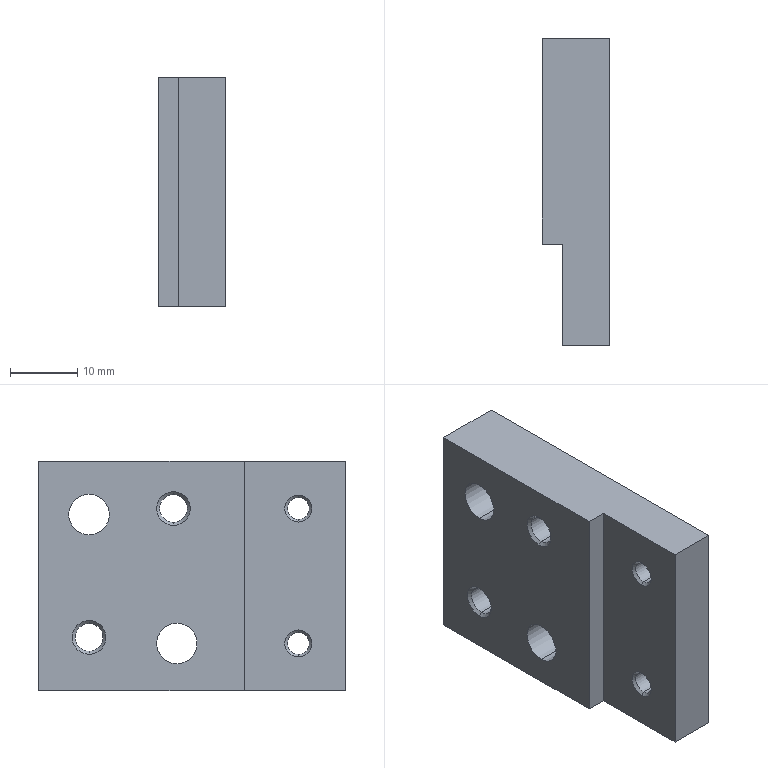Part | SolidWorks | features MirrorStock 1 | 1 solid | 28 faces | box 10 x 45.5 x 34 mm | volume 12986 mm3 | cylinder 12 | cone 8 | plane 8 | commonest cylinder face diameters 3.242 x4 4.134 x4 6 x4
STEP:
#1=CARTESIAN_POINT('',(-38.,7.5,-11.167));
#2=VERTEX_POINT('',#1);
#3=CARTESIAN_POINT('',(-38.,7.5,-7.033));
#4=VERTEX_POINT('',#3);
#5=CARTESIAN_POINT('',(-38.,7.5,-9.1));
#6=DIRECTION('',(-1.,0.,0.));
#7=DIRECTION('',(0.,0.,1.));
#8=AXIS2_PLACEMENT_3D('',#5,#6,#7);
#9=CIRCLE('',#8,2.067);
#10=EDGE_CURVE('',#2,#4,#9,.T.);
#11=ORIENTED_EDGE('',*,*,#10,.F.);
#12=CARTESIAN_POINT('',(-47.567,7.5,-11.167));
#13=VERTEX_POINT('',#12);
#14=CARTESIAN_POINT('',(-38.,7.5,-11.167));
#15=DIRECTION('',(-1.,0.,0.));
#16=VECTOR('',#15,1000.);
#17=LINE('',#14,#16);
#18=EDGE_CURVE('',#2,#13,#17,.T.);
#19=ORIENTED_EDGE('',*,*,#18,.T.);
#20=CARTESIAN_POINT('',(-47.567,7.5,-7.033));
#21=VERTEX_POINT('',#20);
#22=CARTESIAN_POINT('',(-47.567,7.5,-9.1));
#23=DIRECTION('',(-1.,0.,0.));
#24=DIRECTION('',(0.,0.,1.));
#25=AXIS2_PLACEMENT_3D('',#22,#23,#24);
#26=CIRCLE('',#25,2.067);
#27=EDGE_CURVE('',#13,#21,#26,.T.);
#28=ORIENTED_EDGE('',*,*,#27,.T.);
#29=CARTESIAN_POINT('',(-38.,7.5,-7.033));
#30=DIRECTION('',(-1.,0.,0.));
#31=VECTOR('',#30,1000.);
#32=LINE('',#29,#31);
#33=EDGE_CURVE('',#4,#21,#32,.T.);
#34=ORIENTED_EDGE('',*,*,#33,.F.);
#35=EDGE_LOOP('',(#11,#19,#28,#34));
#36=FACE_OUTER_BOUND('',#35,.T.);
#37=CARTESIAN_POINT('',(-38.,7.5,-9.1));
#38=DIRECTION('',(-1.,0.,0.));
#39=DIRECTION('',(0.,0.,1.));
#40=AXIS2_PLACEMENT_3D('',#37,#38,#39);
#41=CYLINDRICAL_SURFACE('',#40,2.067);
#42=ADVANCED_FACE('',(#36),#41,.F.);
#43=CARTESIAN_POINT('',(-47.567,7.5,-9.1));
#44=DIRECTION('',(-1.,0.,0.));
#45=DIRECTION('',(0.,0.,1.));
#46=AXIS2_PLACEMENT_3D('',#43,#44,#45);
#47=CIRCLE('',#46,2.067);
#48=EDGE_CURVE('',#21,#13,#47,.T.);
#49=ORIENTED_EDGE('',*,*,#48,.F.);
#50=CARTESIAN_POINT('',(-48.,7.5,-6.6));
#51=VERTEX_POINT('',#50);
#52=CARTESIAN_POINT('',(-48.,7.5,-6.6));
#53=DIRECTION('',(-0.7071,0.,0.7071));
#54=VECTOR('',#53,1000.);
#55=LINE('',#52,#54);
#56=EDGE_CURVE('',#21,#51,#55,.T.);
#57=ORIENTED_EDGE('',*,*,#56,.T.);
#58=CARTESIAN_POINT('',(-48.,7.5,-11.6));
#59=VERTEX_POINT('',#58);
#60=CARTESIAN_POINT('',(-48.,7.5,-9.1));
#61=DIRECTION('',(-1.,0.,0.));
#62=DIRECTION('',(0.,0.,1.));
#63=AXIS2_PLACEMENT_3D('',#60,#61,#62);
#64=CIRCLE('',#63,2.5);
#65=EDGE_CURVE('',#51,#59,#64,.T.);
#66=ORIENTED_EDGE('',*,*,#65,.T.);
#67=CARTESIAN_POINT('',(-48.,7.5,-11.6));
#68=DIRECTION('',(-0.7071,0.,-0.7071));
#69=VECTOR('',#68,1000.);
#70=LINE('',#67,#69);
#71=EDGE_CURVE('',#13,#59,#70,.T.);
#72=ORIENTED_EDGE('',*,*,#71,.F.);
#73=EDGE_LOOP('',(#49,#57,#66,#72));
#74=FACE_OUTER_BOUND('',#73,.T.);
#75=CARTESIAN_POINT('',(-48.,7.5,-9.1));
#76=DIRECTION('',(-1.,0.,0.));
#77=DIRECTION('',(0.,0.,-1.));
#78=AXIS2_PLACEMENT_3D('',#75,#76,#77);
#79=CONICAL_SURFACE('',#78,2.5,0.7854);
#80=ADVANCED_FACE('',(#74),#79,.F.);
#81=CARTESIAN_POINT('',(-38.,-5.,7.933));
#82=VERTEX_POINT('',#81);
#83=CARTESIAN_POINT('',(-38.,-5.,12.067));
#84=VERTEX_POINT('',#83);
#85=CARTESIAN_POINT('',(-38.,-5.,10.));
#86=DIRECTION('',(-1.,0.,0.));
#87=DIRECTION('',(0.,0.,1.));
#88=AXIS2_PLACEMENT_3D('',#85,#86,#87);
#89=CIRCLE('',#88,2.067);
#90=EDGE_CURVE('',#82,#84,#89,.T.);
#91=ORIENTED_EDGE('',*,*,#90,.F.);
#92=CARTESIAN_POINT('',(-47.567,-5.,7.933));
#93=VERTEX_POINT('',#92);
#94=CARTESIAN_POINT('',(-38.,-5.,7.933));
#95=DIRECTION('',(-1.,0.,0.));
#96=VECTOR('',#95,1000.);
#97=LINE('',#94,#96);
#98=EDGE_CURVE('',#82,#93,#97,.T.);
#99=ORIENTED_EDGE('',*,*,#98,.T.);
#100=CARTESIAN_POINT('',(-47.567,-5.,12.067));
#101=VERTEX_POINT('',#100);
#102=CARTESIAN_POINT('',(-47.567,-5.,10.));
#103=DIRECTION('',(-1.,0.,0.));
#104=DIRECTION('',(0.,0.,1.));
#105=AXIS2_PLACEMENT_3D('',#102,#103,#104);
#106=CIRCLE('',#105,2.067);
#107=EDGE_CURVE('',#93,#101,#106,.T.);
#108=ORIENTED_EDGE('',*,*,#107,.T.);
#109=CARTESIAN_POINT('',(-38.,-5.,12.067));
#110=DIRECTION('',(-1.,0.,0.));
#111=VECTOR('',#110,1000.);
#112=LINE('',#109,#111);
#113=EDGE_CURVE('',#84,#101,#112,.T.);
#114=ORIENTED_EDGE('',*,*,#113,.F.);
#115=EDGE_LOOP('',(#91,#99,#108,#114));
#116=FACE_OUTER_BOUND('',#115,.T.);
#117=CARTESIAN_POINT('',(-38.,-5.,10.));
#118=DIRECTION('',(-1.,0.,0.));
#119=DIRECTION('',(0.,0.,1.));
#120=AXIS2_PLACEMENT_3D('',#117,#118,#119);
#121=CYLINDRICAL_SURFACE('',#120,2.067);
#122=ADVANCED_FACE('',(#116),#121,.F.);
#123=CARTESIAN_POINT('',(-47.567,-5.,10.));
#124=DIRECTION('',(-1.,0.,0.));
#125=DIRECTION('',(0.,0.,1.));
#126=AXIS2_PLACEMENT_3D('',#123,#124,#125);
#127=CIRCLE('',#126,2.067);
#128=EDGE_CURVE('',#101,#93,#127,.T.);
#129=ORIENTED_EDGE('',*,*,#128,.F.);
#130=CARTESIAN_POINT('',(-48.,-5.,12.5));
#131=VERTEX_POINT('',#130);
#132=CARTESIAN_POINT('',(-48.,-5.,12.5));
#133=DIRECTION('',(-0.7071,0.,0.7071));
#134=VECTOR('',#133,1000.);
#135=LINE('',#132,#134);
#136=EDGE_CURVE('',#101,#131,#135,.T.);
#137=ORIENTED_EDGE('',*,*,#136,.T.);
#138=CARTESIAN_POINT('',(-48.,-5.,7.5));
#139=VERTEX_POINT('',#138);
#140=CARTESIAN_POINT('',(-48.,-5.,10.));
#141=DIRECTION('',(-1.,0.,0.));
#142=DIRECTION('',(0.,0.,1.));
#143=AXIS2_PLACEMENT_3D('',#140,#141,#142);
#144=CIRCLE('',#143,2.5);
#145=EDGE_CURVE('',#131,#139,#144,.T.);
#146=ORIENTED_EDGE('',*,*,#145,.T.);
#147=CARTESIAN_POINT('',(-48.,-5.,7.5));
#148=DIRECTION('',(-0.7071,0.,-0.7071));
#149=VECTOR('',#148,1000.);
#150=LINE('',#147,#149);
#151=EDGE_CURVE('',#93,#139,#150,.T.);
#152=ORIENTED_EDGE('',*,*,#151,.F.);
#153=EDGE_LOOP('',(#129,#137,#146,#152));
#154=FACE_OUTER_BOUND('',#153,.T.);
#155=CARTESIAN_POINT('',(-48.,-5.,10.));
#156=DIRECTION('',(-1.,0.,0.));
#157=DIRECTION('',(0.,0.,-1.));
#158=AXIS2_PLACEMENT_3D('',#155,#156,#157);
#159=CONICAL_SURFACE('',#158,2.5,0.7854);
#160=ADVANCED_FACE('',(#154),#159,.F.);
#161=CARTESIAN_POINT('',(-38.,-23.5,11.621));
#162=VERTEX_POINT('',#161);
#163=CARTESIAN_POINT('',(-38.,-23.5,8.379));
#164=VERTEX_POINT('',#163);
#165=CARTESIAN_POINT('',(-38.,-23.5,10.));
#166=DIRECTION('',(1.,0.,0.));
#167=DIRECTION('',(0.,0.,1.));
#168=AXIS2_PLACEMENT_3D('',#165,#166,#167);
#169=CIRCLE('',#168,1.621);
#170=EDGE_CURVE('',#162,#164,#169,.T.);
#171=ORIENTED_EDGE('',*,*,#170,.T.);
#172=CARTESIAN_POINT('',(-44.621,-23.5,8.379));
#173=VERTEX_POINT('',#172);
#174=CARTESIAN_POINT('',(-35.,-23.5,8.379));
#175=DIRECTION('',(-1.,0.,0.));
#176=VECTOR('',#175,1000.);
#177=LINE('',#174,#176);
#178=EDGE_CURVE('',#164,#173,#177,.T.);
#179=ORIENTED_EDGE('',*,*,#178,.T.);
#180=CARTESIAN_POINT('',(-44.621,-23.5,11.621));
#181=VERTEX_POINT('',#180);
#182=CARTESIAN_POINT('',(-44.621,-23.5,10.));
#183=DIRECTION('',(-1.,0.,0.));
#184=DIRECTION('',(0.,0.,1.));
#185=AXIS2_PLACEMENT_3D('',#182,#183,#184);
#186=CIRCLE('',#185,1.621);
#187=EDGE_CURVE('',#173,#181,#186,.T.);
#188=ORIENTED_EDGE('',*,*,#187,.T.);
#189=CARTESIAN_POINT('',(-35.,-23.5,11.621));
#190=DIRECTION('',(-1.,0.,0.));
#191=VECTOR('',#190,1000.);
#192=LINE('',#189,#191);
#193=EDGE_CURVE('',#162,#181,#192,.T.);
#194=ORIENTED_EDGE('',*,*,#193,.F.);
#195=EDGE_LOOP('',(#171,#179,#188,#194));
#196=FACE_OUTER_BOUND('',#195,.T.);
#197=CARTESIAN_POINT('',(-35.,-23.5,10.));
#198=DIRECTION('',(-1.,0.,0.));
#199=DIRECTION('',(0.,0.,1.));
#200=AXIS2_PLACEMENT_3D('',#197,#198,#199);
#201=CYLINDRICAL_SURFACE('',#200,1.621);
#202=ADVANCED_FACE('',(#196),#201,.F.);
#203=CARTESIAN_POINT('',(-44.621,-23.5,10.));
#204=DIRECTION('',(-1.,0.,0.));
#205=DIRECTION('',(0.,0.,1.));
#206=AXIS2_PLACEMENT_3D('',#203,#204,#205);
#207=CIRCLE('',#206,1.621);
#208=EDGE_CURVE('',#181,#173,#207,.T.);
#209=ORIENTED_EDGE('',*,*,#208,.F.);
#210=CARTESIAN_POINT('',(-45.,-23.5,12.));
#211=VERTEX_POINT('',#210);
#212=CARTESIAN_POINT('',(-45.,-23.5,12.));
#213=DIRECTION('',(-0.7071,0.,0.7071));
#214=VECTOR('',#213,1000.);
#215=LINE('',#212,#214);
#216=EDGE_CURVE('',#181,#211,#215,.T.);
#217=ORIENTED_EDGE('',*,*,#216,.T.);
#218=CARTESIAN_POINT('',(-45.,-23.5,8.));
#219=VERTEX_POINT('',#218);
#220=CARTESIAN_POINT('',(-45.,-23.5,10.));
#221=DIRECTION('',(-1.,0.,0.));
#222=DIRECTION('',(0.,0.,1.));
#223=AXIS2_PLACEMENT_3D('',#220,#221,#222);
#224=CIRCLE('',#223,2.);
#225=EDGE_CURVE('',#211,#219,#224,.T.);
#226=ORIENTED_EDGE('',*,*,#225,.T.);
#227=CARTESIAN_POINT('',(-45.,-23.5,8.));
#228=DIRECTION('',(-0.7071,0.,-0.7071));
#229=VECTOR('',#228,1000.);
#230=LINE('',#227,#229);
#231=EDGE_CURVE('',#173,#219,#230,.T.);
#232=ORIENTED_EDGE('',*,*,#231,.F.);
#233=EDGE_LOOP('',(#209,#217,#226,#232));
#234=FACE_OUTER_BOUND('',#233,.T.);
#235=CARTESIAN_POINT('',(-45.,-23.5,10.));
#236=DIRECTION('',(-1.,0.,0.));
#237=DIRECTION('',(0.,0.,-1.));
#238=AXIS2_PLACEMENT_3D('',#235,#236,#237);
#239=CONICAL_SURFACE('',#238,2.,0.7854);
#240=ADVANCED_FACE('',(#234),#239,.F.);
#241=CARTESIAN_POINT('',(-44.621,-23.5,-8.379));
#242=VERTEX_POINT('',#241);
#243=CARTESIAN_POINT('',(-44.621,-23.5,-11.621));
#244=VERTEX_POINT('',#243);
#245=CARTESIAN_POINT('',(-44.621,-23.5,-10.));
#246=DIRECTION('',(-1.,0.,0.));
#247=DIRECTION('',(0.,0.,1.));
#248=AXIS2_PLACEMENT_3D('',#245,#246,#247);
#249=CIRCLE('',#248,1.621);
#250=EDGE_CURVE('',#242,#244,#249,.T.);
#251=ORIENTED_EDGE('',*,*,#250,.F.);
#252=CARTESIAN_POINT('',(-45.,-23.5,-8.));
#253=VERTEX_POINT('',#252);
#254=CARTESIAN_POINT('',(-45.,-23.5,-8.));
#255=DIRECTION('',(-0.7071,0.,0.7071));
#256=VECTOR('',#255,1000.);
#257=LINE('',#254,#256);
#258=EDGE_CURVE('',#242,#253,#257,.T.);
#259=ORIENTED_EDGE('',*,*,#258,.T.);
#260=CARTESIAN_POINT('',(-45.,-23.5,-12.));
#261=VERTEX_POINT('',#260);
#262=CARTESIAN_POINT('',(-45.,-23.5,-10.));
#263=DIRECTION('',(-1.,0.,0.));
#264=DIRECTION('',(0.,0.,1.));
#265=AXIS2_PLACEMENT_3D('',#262,#263,#264);
#266=CIRCLE('',#265,2.);
#267=EDGE_CURVE('',#253,#261,#266,.T.);
#268=ORIENTED_EDGE('',*,*,#267,.T.);
#269=CARTESIAN_POINT('',(-45.,-23.5,-12.));
#270=DIRECTION('',(-0.7071,0.,-0.7071));
#271=VECTOR('',#270,1000.);
#272=LINE('',#269,#271);
#273=EDGE_CURVE('',#244,#261,#272,.T.);
#274=ORIENTED_EDGE('',*,*,#273,.F.);
#275=EDGE_LOOP('',(#251,#259,#268,#274));
#276=FACE_OUTER_BOUND('',#275,.T.);
#277=CARTESIAN_POINT('',(-45.,-23.5,-10.));
#278=DIRECTION('',(-1.,0.,0.));
#279=DIRECTION('',(0.,0.,-1.));
#280=AXIS2_PLACEMENT_3D('',#277,#278,#279);
#281=CONICAL_SURFACE('',#280,2.,0.7854);
#282=ADVANCED_FACE('',(#276),#281,.F.);
#283=CARTESIAN_POINT('',(-38.,-5.5,-13.));
#284=VERTEX_POINT('',#283);
#285=CARTESIAN_POINT('',(-38.,-5.5,-7.));
#286=VERTEX_POINT('',#285);
#287=CARTESIAN_POINT('',(-38.,-5.5,-10.));
#288=DIRECTION('',(-1.,0.,0.));
#289=DIRECTION('',(0.,0.,1.));
#290=AXIS2_PLACEMENT_3D('',#287,#288,#289);
#291=CIRCLE('',#290,3.);
#292=EDGE_CURVE('',#284,#286,#291,.T.);
#293=ORIENTED_EDGE('',*,*,#292,.F.);
#294=CARTESIAN_POINT('',(-48.,-5.5,-13.));
#295=VERTEX_POINT('',#294);
#296=CARTESIAN_POINT('',(-100.,-5.5,-13.));
#297=DIRECTION('',(-1.,0.,0.));
#298=VECTOR('',#297,1000.);
#299=LINE('',#296,#298);
#300=EDGE_CURVE('',#284,#295,#299,.T.);
#301=ORIENTED_EDGE('',*,*,#300,.T.);
#302=CARTESIAN_POINT('',(-48.,-5.5,-7.));
#303=VERTEX_POINT('',#302);
#304=CARTESIAN_POINT('',(-48.,-5.5,-10.));
#305=DIRECTION('',(-1.,0.,0.));
#306=DIRECTION('',(0.,0.,1.));
#307=AXIS2_PLACEMENT_3D('',#304,#305,#306);
#308=CIRCLE('',#307,3.);
#309=EDGE_CURVE('',#295,#303,#308,.T.);
#310=ORIENTED_EDGE('',*,*,#309,.T.);
#311=CARTESIAN_POINT('',(-100.,-5.5,-7.));
#312=DIRECTION('',(-1.,0.,0.));
#313=VECTOR('',#312,1000.);
#314=LINE('',#311,#313);
#315=EDGE_CURVE('',#286,#303,#314,.T.);
#316=ORIENTED_EDGE('',*,*,#315,.F.);
#317=EDGE_LOOP('',(#293,#301,#310,#316));
#318=FACE_OUTER_BOUND('',#317,.T.);
#319=CARTESIAN_POINT('',(-100.,-5.5,-10.));
#320=DIRECTION('',(-1.,0.,0.));
#321=DIRECTION('',(0.,0.,1.));
#322=AXIS2_PLACEMENT_3D('',#319,#320,#321);
#323=CYLINDRICAL_SURFACE('',#322,3.);
#324=ADVANCED_FACE('',(#318),#323,.F.);
#325=CARTESIAN_POINT('',(-38.,7.5,6.1));
#326=VERTEX_POINT('',#325);
#327=CARTESIAN_POINT('',(-38.,7.5,12.1));
#328=VERTEX_POINT('',#327);
#329=CARTESIAN_POINT('',(-38.,7.5,9.1));
#330=DIRECTION('',(-1.,0.,0.));
#331=DIRECTION('',(0.,0.,1.));
#332=AXIS2_PLACEMENT_3D('',#329,#330,#331);
#333=CIRCLE('',#332,3.);
#334=EDGE_CURVE('',#326,#328,#333,.T.);
#335=ORIENTED_EDGE('',*,*,#334,.F.);
#336=CARTESIAN_POINT('',(-48.,7.5,6.1));
#337=VERTEX_POINT('',#336);
#338=CARTESIAN_POINT('',(-100.,7.5,6.1));
#339=DIRECTION('',(-1.,0.,0.));
#340=VECTOR('',#339,1000.);
#341=LINE('',#338,#340);
#342=EDGE_CURVE('',#326,#337,#341,.T.);
#343=ORIENTED_EDGE('',*,*,#342,.T.);
#344=CARTESIAN_POINT('',(-48.,7.5,12.1));
#345=VERTEX_POINT('',#344);
#346=CARTESIAN_POINT('',(-48.,7.5,9.1));
#347=DIRECTION('',(-1.,0.,0.));
#348=DIRECTION('',(0.,0.,1.));
#349=AXIS2_PLACEMENT_3D('',#346,#347,#348);
#350=CIRCLE('',#349,3.);
#351=EDGE_CURVE('',#337,#345,#350,.T.);
#352=ORIENTED_EDGE('',*,*,#351,.T.);
#353=CARTESIAN_POINT('',(-100.,7.5,12.1));
#354=DIRECTION('',(-1.,0.,0.));
#355=VECTOR('',#354,1000.);
#356=LINE('',#353,#355);
#357=EDGE_CURVE('',#328,#345,#356,.T.);
#358=ORIENTED_EDGE('',*,*,#357,.F.);
#359=EDGE_LOOP('',(#335,#343,#352,#358));
#360=FACE_OUTER_BOUND('',#359,.T.);
#361=CARTESIAN_POINT('',(-100.,7.5,9.1));
#362=DIRECTION('',(-1.,0.,0.));
#363=DIRECTION('',(0.,0.,1.));
#364=AXIS2_PLACEMENT_3D('',#361,#362,#363);
#365=CYLINDRICAL_SURFACE('',#364,3.);
#366=ADVANCED_FACE('',(#360),#365,.F.);
#367=CARTESIAN_POINT('',(-38.,-23.5,-8.379));
#368=VERTEX_POINT('',#367);
#369=CARTESIAN_POINT('',(-38.,-23.5,-11.621));
#370=VERTEX_POINT('',#369);
#371=CARTESIAN_POINT('',(-38.,-23.5,-10.));
#372=DIRECTION('',(1.,0.,0.));
#373=DIRECTION('',(0.,0.,1.));
#374=AXIS2_PLACEMENT_3D('',#371,#372,#373);
#375=CIRCLE('',#374,1.621);
#376=EDGE_CURVE('',#368,#370,#375,.T.);
#377=ORIENTED_EDGE('',*,*,#376,.T.);
#378=CARTESIAN_POINT('',(-35.,-23.5,-11.621));
#379=DIRECTION('',(-1.,0.,0.));
#380=VECTOR('',#379,1000.);
#381=LINE('',#378,#380);
#382=EDGE_CURVE('',#370,#244,#381,.T.);
#383=ORIENTED_EDGE('',*,*,#382,.T.);
#384=CARTESIAN_POINT('',(-44.621,-23.5,-10.));
#385=DIRECTION('',(-1.,0.,0.));
#386=DIRECTION('',(0.,0.,1.));
#387=AXIS2_PLACEMENT_3D('',#384,#385,#386);
#388=CIRCLE('',#387,1.621);
#389=EDGE_CURVE('',#244,#242,#388,.T.);
#390=ORIENTED_EDGE('',*,*,#389,.T.);
#391=CARTESIAN_POINT('',(-35.,-23.5,-8.379));
#392=DIRECTION('',(-1.,0.,0.));
#393=VECTOR('',#392,1000.);
#394=LINE('',#391,#393);
#395=EDGE_CURVE('',#368,#242,#394,.T.);
#396=ORIENTED_EDGE('',*,*,#395,.F.);
#397=EDGE_LOOP('',(#377,#383,#390,#396));
#398=FACE_OUTER_BOUND('',#397,.T.);
#399=CARTESIAN_POINT('',(-35.,-23.5,-10.));
#400=DIRECTION('',(-1.,0.,0.));
#401=DIRECTION('',(0.,0.,1.));
#402=AXIS2_PLACEMENT_3D('',#399,#400,#401);
#403=CYLINDRICAL_SURFACE('',#402,1.621);
#404=ADVANCED_FACE('',(#398),#403,.F.);
#405=ORIENTED_EDGE('',*,*,#382,.F.);
#406=CARTESIAN_POINT('',(-38.,-23.5,-10.));
#407=DIRECTION('',(1.,0.,0.));
#408=DIRECTION('',(0.,0.,1.));
#409=AXIS2_PLACEMENT_3D('',#406,#407,#408);
#410=CIRCLE('',#409,1.621);
#411=EDGE_CURVE('',#370,#368,#410,.T.);
#412=ORIENTED_EDGE('',*,*,#411,.T.);
#413=ORIENTED_EDGE('',*,*,#395,.T.);
#414=ORIENTED_EDGE('',*,*,#250,.T.);
#415=EDGE_LOOP('',(#405,#412,#413,#414));
#416=FACE_OUTER_BOUND('',#415,.T.);
#417=CARTESIAN_POINT('',(-35.,-23.5,-10.));
#418=DIRECTION('',(-1.,0.,0.));
#419=DIRECTION('',(0.,0.,1.));
#420=AXIS2_PLACEMENT_3D('',#417,#418,#419);
#421=CYLINDRICAL_SURFACE('',#420,1.621);
#422=ADVANCED_FACE('',(#416),#421,.F.);
#423=CARTESIAN_POINT('',(-45.,-30.5,-17.));
#424=VERTEX_POINT('',#423);
#425=CARTESIAN_POINT('',(-45.,-30.5,17.));
#426=VERTEX_POINT('',#425);
#427=CARTESIAN_POINT('',(-45.,-30.5,-17.));
#428=DIRECTION('',(0.,0.,1.));
#429=VECTOR('',#428,1000.);
#430=LINE('',#427,#429);
#431=EDGE_CURVE('',#424,#426,#430,.T.);
#432=ORIENTED_EDGE('',*,*,#431,.F.);
#433=CARTESIAN_POINT('',(-38.,-30.5,-17.));
#434=VERTEX_POINT('',#433);
#435=CARTESIAN_POINT('',(-48.,-30.5,-17.));
#436=DIRECTION('',(1.,0.,0.));
#437=VECTOR('',#436,1000.);
#438=LINE('',#435,#437);
#439=EDGE_CURVE('',#424,#434,#438,.T.);
#440=ORIENTED_EDGE('',*,*,#439,.T.);
#441=CARTESIAN_POINT('',(-38.,-30.5,17.));
#442=VERTEX_POINT('',#441);
#443=CARTESIAN_POINT('',(-38.,-30.5,-17.));
#444=DIRECTION('',(0.,0.,1.));
#445=VECTOR('',#444,1000.);
#446=LINE('',#443,#445);
#447=EDGE_CURVE('',#434,#442,#446,.T.);
#448=ORIENTED_EDGE('',*,*,#447,.T.);
#449=CARTESIAN_POINT('',(-48.,-30.5,17.));
#450=DIRECTION('',(1.,0.,0.));
#451=VECTOR('',#450,1000.);
#452=LINE('',#449,#451);
#453=EDGE_CURVE('',#426,#442,#452,.T.);
#454=ORIENTED_EDGE('',*,*,#453,.F.);
#455=EDGE_LOOP('',(#432,#440,#448,#454));
#456=FACE_OUTER_BOUND('',#455,.T.);
#457=CARTESIAN_POINT('',(-48.,-30.5,-17.));
#458=DIRECTION('',(0.,-1.,0.));
#459=DIRECTION('',(0.,0.,1.));
#460=AXIS2_PLACEMENT_3D('',#457,#458,#459);
#461=PLANE('',#460);
#462=ADVANCED_FACE('',(#456),#461,.T.);
#463=CARTESIAN_POINT('',(-38.,15.,17.));
#464=VERTEX_POINT('',#463);
#465=CARTESIAN_POINT('',(-38.,15.,-17.));
#466=VERTEX_POINT('',#465);
#467=CARTESIAN_POINT('',(-38.,15.,17.));
#468=DIRECTION('',(0.,0.,-1.));
#469=VECTOR('',#468,1000.);
#470=LINE('',#467,#469);
#471=EDGE_CURVE('',#464,#466,#470,.T.);
#472=ORIENTED_EDGE('',*,*,#471,.T.);
#473=CARTESIAN_POINT('',(-48.,15.,-17.));
#474=VERTEX_POINT('',#473);
#475=CARTESIAN_POINT('',(-48.,15.,-17.));
#476=DIRECTION('',(1.,0.,0.));
#477=VECTOR('',#476,1000.);
#478=LINE('',#475,#477);
#479=EDGE_CURVE('',#474,#466,#478,.T.);
#480=ORIENTED_EDGE('',*,*,#479,.F.);
#481=CARTESIAN_POINT('',(-48.,15.,17.));
#482=VERTEX_POINT('',#481);
#483=CARTESIAN_POINT('',(-48.,15.,17.));
#484=DIRECTION('',(0.,0.,-1.));
#485=VECTOR('',#484,1000.);
#486=LINE('',#483,#485);
#487=EDGE_CURVE('',#482,#474,#486,.T.);
#488=ORIENTED_EDGE('',*,*,#487,.F.);
#489=CARTESIAN_POINT('',(-48.,15.,17.));
#490=DIRECTION('',(1.,0.,0.));
#491=VECTOR('',#490,1000.);
#492=LINE('',#489,#491);
#493=EDGE_CURVE('',#482,#464,#492,.T.);
#494=ORIENTED_EDGE('',*,*,#493,.T.);
#495=EDGE_LOOP('',(#472,#480,#488,#494));
#496=FACE_OUTER_BOUND('',#495,.T.);
#497=CARTESIAN_POINT('',(-48.,15.,17.));
#498=DIRECTION('',(0.,1.,0.));
#499=DIRECTION('',(1.,0.,0.));
#500=AXIS2_PLACEMENT_3D('',#497,#498,#499);
#501=PLANE('',#500);
#502=ADVANCED_FACE('',(#496),#501,.T.);
#503=CARTESIAN_POINT('',(-48.,-15.5,17.));
#504=VERTEX_POINT('',#503);
#505=CARTESIAN_POINT('',(-48.,-15.5,-17.));
#506=VERTEX_POINT('',#505);
#507=CARTESIAN_POINT('',(-48.,-15.5,17.));
#508=DIRECTION('',(0.,0.,-1.));
#509=VECTOR('',#508,1000.);
#510=LINE('',#507,#509);
#511=EDGE_CURVE('',#504,#506,#510,.T.);
#512=ORIENTED_EDGE('',*,*,#511,.F.);
#513=CARTESIAN_POINT('',(-48.,-30.5,17.));
#514=DIRECTION('',(0.,1.,0.));
#515=VECTOR('',#514,1000.);
#516=LINE('',#513,#515);
#517=EDGE_CURVE('',#504,#482,#516,.T.);
#518=ORIENTED_EDGE('',*,*,#517,.T.);
#519=ORIENTED_EDGE('',*,*,#487,.T.);
#520=CARTESIAN_POINT('',(-48.,15.,-17.));
#521=DIRECTION('',(0.,-1.,0.));
#522=VECTOR('',#521,1000.);
#523=LINE('',#520,#522);
#524=EDGE_CURVE('',#474,#506,#523,.T.);
#525=ORIENTED_EDGE('',*,*,#524,.T.);
#526=EDGE_LOOP('',(#512,#518,#519,#525));
#527=FACE_OUTER_BOUND('',#526,.T.);
#528=CARTESIAN_POINT('',(-48.,7.5,-9.1));
#529=DIRECTION('',(-1.,0.,0.));
#530=DIRECTION('',(0.,0.,1.));
#531=AXIS2_PLACEMENT_3D('',#528,#529,#530);
#532=CIRCLE('',#531,2.5);
#533=EDGE_CURVE('',#59,#51,#532,.T.);
#534=ORIENTED_EDGE('',*,*,#533,.F.);
#535=ORIENTED_EDGE('',*,*,#65,.F.);
#536=EDGE_LOOP('',(#534,#535));
#537=FACE_BOUND('',#536,.T.);
#538=CARTESIAN_POINT('',(-48.,-5.,10.));
#539=DIRECTION('',(-1.,0.,0.));
#540=DIRECTION('',(0.,0.,1.));
#541=AXIS2_PLACEMENT_3D('',#538,#539,#540);
#542=CIRCLE('',#541,2.5);
#543=EDGE_CURVE('',#139,#131,#542,.T.);
#544=ORIENTED_EDGE('',*,*,#543,.F.);
#545=ORIENTED_EDGE('',*,*,#145,.F.);
#546=EDGE_LOOP('',(#544,#545));
#547=FACE_BOUND('',#546,.T.);
#548=CARTESIAN_POINT('',(-48.,-5.5,-10.));
#549=DIRECTION('',(-1.,0.,0.));
#550=DIRECTION('',(0.,0.,1.));
#551=AXIS2_PLACEMENT_3D('',#548,#549,#550);
#552=CIRCLE('',#551,3.);
#553=EDGE_CURVE('',#303,#295,#552,.T.);
#554=ORIENTED_EDGE('',*,*,#553,.F.);
#555=ORIENTED_EDGE('',*,*,#309,.F.);
#556=EDGE_LOOP('',(#554,#555));
#557=FACE_BOUND('',#556,.T.);
#558=CARTESIAN_POINT('',(-48.,7.5,9.1));
#559=DIRECTION('',(-1.,0.,0.));
#560=DIRECTION('',(0.,0.,1.));
#561=AXIS2_PLACEMENT_3D('',#558,#559,#560);
#562=CIRCLE('',#561,3.);
#563=EDGE_CURVE('',#345,#337,#562,.T.);
#564=ORIENTED_EDGE('',*,*,#563,.F.);
#565=ORIENTED_EDGE('',*,*,#351,.F.);
#566=EDGE_LOOP('',(#564,#565));
#567=FACE_BOUND('',#566,.T.);
#568=CARTESIAN_POINT('',(-48.,0.,0.));
#569=DIRECTION('',(1.,0.,0.));
#570=DIRECTION('',(0.,1.,0.));
#571=AXIS2_PLACEMENT_3D('',#568,#569,#570);
#572=PLANE('',#571);
#573=ADVANCED_FACE('',(#527,#537,#547,#557,#567),#572,.F.);
#574=ORIENTED_EDGE('',*,*,#524,.F.);
#575=ORIENTED_EDGE('',*,*,#479,.T.);
#576=CARTESIAN_POINT('',(-38.,15.,-17.));
#577=DIRECTION('',(0.,-1.,0.));
#578=VECTOR('',#577,1000.);
#579=LINE('',#576,#578);
#580=EDGE_CURVE('',#466,#434,#579,.T.);
#581=ORIENTED_EDGE('',*,*,#580,.T.);
#582=ORIENTED_EDGE('',*,*,#439,.F.);
#583=CARTESIAN_POINT('',(-45.,-15.5,-17.));
#584=VERTEX_POINT('',#583);
#585=CARTESIAN_POINT('',(-45.,-15.5,-17.));
#586=DIRECTION('',(0.,-1.,0.));
#587=VECTOR('',#586,1000.);
#588=LINE('',#585,#587);
#589=EDGE_CURVE('',#584,#424,#588,.T.);
#590=ORIENTED_EDGE('',*,*,#589,.F.);
#591=CARTESIAN_POINT('',(-45.,-15.5,-17.));
#592=DIRECTION('',(-1.,0.,0.));
#593=VECTOR('',#592,1000.);
#594=LINE('',#591,#593);
#595=EDGE_CURVE('',#584,#506,#594,.T.);
#596=ORIENTED_EDGE('',*,*,#595,.T.);
#597=EDGE_LOOP('',(#574,#575,#581,#582,#590,#596));
#598=FACE_OUTER_BOUND('',#597,.T.);
#599=CARTESIAN_POINT('',(-48.,15.,-17.));
#600=DIRECTION('',(0.,0.,-1.));
#601=DIRECTION('',(1.,0.,0.));
#602=AXIS2_PLACEMENT_3D('',#599,#600,#601);
#603=PLANE('',#602);
#604=ADVANCED_FACE('',(#598),#603,.T.);
#605=CARTESIAN_POINT('',(-45.,-15.5,17.));
#606=VERTEX_POINT('',#605);
#607=CARTESIAN_POINT('',(-45.,-30.5,17.));
#608=DIRECTION('',(0.,1.,0.));
#609=VECTOR('',#608,1000.);
#610=LINE('',#607,#609);
#611=EDGE_CURVE('',#426,#606,#610,.T.);
#612=ORIENTED_EDGE('',*,*,#611,.F.);
#613=ORIENTED_EDGE('',*,*,#453,.T.);
#614=CARTESIAN_POINT('',(-38.,-30.5,17.));
#615=DIRECTION('',(0.,1.,0.));
#616=VECTOR('',#615,1000.);
#617=LINE('',#614,#616);
#618=EDGE_CURVE('',#442,#464,#617,.T.);
#619=ORIENTED_EDGE('',*,*,#618,.T.);
#620=ORIENTED_EDGE('',*,*,#493,.F.);
#621=ORIENTED_EDGE('',*,*,#517,.F.);
#622=CARTESIAN_POINT('',(-45.,-15.5,17.));
#623=DIRECTION('',(-1.,0.,0.));
#624=VECTOR('',#623,1000.);
#625=LINE('',#622,#624);
#626=EDGE_CURVE('',#606,#504,#625,.T.);
#627=ORIENTED_EDGE('',*,*,#626,.F.);
#628=EDGE_LOOP('',(#612,#613,#619,#620,#621,#627));
#629=FACE_OUTER_BOUND('',#628,.T.);
#630=CARTESIAN_POINT('',(-48.,-30.5,17.));
#631=DIRECTION('',(0.,0.,1.));
#632=DIRECTION('',(0.,-1.,0.));
#633=AXIS2_PLACEMENT_3D('',#630,#631,#632);
#634=PLANE('',#633);
#635=ADVANCED_FACE('',(#629),#634,.T.);
#636=ORIENTED_EDGE('',*,*,#580,.F.);
#637=ORIENTED_EDGE('',*,*,#471,.F.);
#638=ORIENTED_EDGE('',*,*,#618,.F.);
#639=ORIENTED_EDGE('',*,*,#447,.F.);
#640=EDGE_LOOP('',(#636,#637,#638,#639));
#641=FACE_OUTER_BOUND('',#640,.T.);
#642=CARTESIAN_POINT('',(-38.,7.5,-9.1));
#643=DIRECTION('',(-1.,0.,0.));
#644=DIRECTION('',(0.,0.,1.));
#645=AXIS2_PLACEMENT_3D('',#642,#643,#644);
#646=CIRCLE('',#645,2.067);
#647=EDGE_CURVE('',#4,#2,#646,.T.);
#648=ORIENTED_EDGE('',*,*,#647,.T.);
#649=ORIENTED_EDGE('',*,*,#10,.T.);
#650=EDGE_LOOP('',(#648,#649));
#651=FACE_BOUND('',#650,.T.);
#652=CARTESIAN_POINT('',(-38.,-5.,10.));
#653=DIRECTION('',(-1.,0.,0.));
#654=DIRECTION('',(0.,0.,1.));
#655=AXIS2_PLACEMENT_3D('',#652,#653,#654);
#656=CIRCLE('',#655,2.067);
#657=EDGE_CURVE('',#84,#82,#656,.T.);
#658=ORIENTED_EDGE('',*,*,#657,.T.);
#659=ORIENTED_EDGE('',*,*,#90,.T.);
#660=EDGE_LOOP('',(#658,#659));
#661=FACE_BOUND('',#660,.T.);
#662=ORIENTED_EDGE('',*,*,#170,.F.);
#663=CARTESIAN_POINT('',(-38.,-23.5,10.));
#664=DIRECTION('',(1.,0.,0.));
#665=DIRECTION('',(0.,0.,1.));
#666=AXIS2_PLACEMENT_3D('',#663,#664,#665);
#667=CIRCLE('',#666,1.621);
#668=EDGE_CURVE('',#164,#162,#667,.T.);
#669=ORIENTED_EDGE('',*,*,#668,.F.);
#670=EDGE_LOOP('',(#662,#669));
#671=FACE_BOUND('',#670,.T.);
#672=ORIENTED_EDGE('',*,*,#376,.F.);
#673=ORIENTED_EDGE('',*,*,#411,.F.);
#674=EDGE_LOOP('',(#672,#673));
#675=FACE_BOUND('',#674,.T.);
#676=CARTESIAN_POINT('',(-38.,-5.5,-10.));
#677=DIRECTION('',(-1.,0.,0.));
#678=DIRECTION('',(0.,0.,1.));
#679=AXIS2_PLACEMENT_3D('',#676,#677,#678);
#680=CIRCLE('',#679,3.);
#681=EDGE_CURVE('',#286,#284,#680,.T.);
#682=ORIENTED_EDGE('',*,*,#681,.T.);
#683=ORIENTED_EDGE('',*,*,#292,.T.);
#684=EDGE_LOOP('',(#682,#683));
#685=FACE_BOUND('',#684,.T.);
#686=CARTESIAN_POINT('',(-38.,7.5,9.1));
#687=DIRECTION('',(-1.,0.,0.));
#688=DIRECTION('',(0.,0.,1.));
#689=AXIS2_PLACEMENT_3D('',#686,#687,#688);
#690=CIRCLE('',#689,3.);
#691=EDGE_CURVE('',#328,#326,#690,.T.);
#692=ORIENTED_EDGE('',*,*,#691,.T.);
#693=ORIENTED_EDGE('',*,*,#334,.T.);
#694=EDGE_LOOP('',(#692,#693));
#695=FACE_BOUND('',#694,.T.);
#696=CARTESIAN_POINT('',(-38.,0.,0.));
#697=DIRECTION('',(1.,0.,0.));
#698=DIRECTION('',(0.,1.,0.));
#699=AXIS2_PLACEMENT_3D('',#696,#697,#698);
#700=PLANE('',#699);
#701=ADVANCED_FACE('',(#641,#651,#661,#671,#675,#685,#695),#700,.T.);
#702=ORIENTED_EDGE('',*,*,#511,.T.);
#703=ORIENTED_EDGE('',*,*,#595,.F.);
#704=CARTESIAN_POINT('',(-45.,-15.5,17.));
#705=DIRECTION('',(0.,0.,-1.));
#706=VECTOR('',#705,1000.);
#707=LINE('',#704,#706);
#708=EDGE_CURVE('',#606,#584,#707,.T.);
#709=ORIENTED_EDGE('',*,*,#708,.F.);
#710=ORIENTED_EDGE('',*,*,#626,.T.);
#711=EDGE_LOOP('',(#702,#703,#709,#710));
#712=FACE_OUTER_BOUND('',#711,.T.);
#713=CARTESIAN_POINT('',(-45.,-15.5,17.));
#714=DIRECTION('',(0.,-1.,0.));
#715=DIRECTION('',(0.,0.,1.));
#716=AXIS2_PLACEMENT_3D('',#713,#714,#715);
#717=PLANE('',#716);
#718=ADVANCED_FACE('',(#712),#717,.T.);
#719=ORIENTED_EDGE('',*,*,#589,.T.);
#720=ORIENTED_EDGE('',*,*,#431,.T.);
#721=ORIENTED_EDGE('',*,*,#611,.T.);
#722=ORIENTED_EDGE('',*,*,#708,.T.);
#723=EDGE_LOOP('',(#719,#720,#721,#722));
#724=FACE_OUTER_BOUND('',#723,.T.);
#725=CARTESIAN_POINT('',(-45.,-23.5,10.));
#726=DIRECTION('',(-1.,0.,0.));
#727=DIRECTION('',(0.,0.,1.));
#728=AXIS2_PLACEMENT_3D('',#725,#726,#727);
#729=CIRCLE('',#728,2.);
#730=EDGE_CURVE('',#219,#211,#729,.T.);
#731=ORIENTED_EDGE('',*,*,#730,.F.);
#732=ORIENTED_EDGE('',*,*,#225,.F.);
#733=EDGE_LOOP('',(#731,#732));
#734=FACE_BOUND('',#733,.T.);
#735=CARTESIAN_POINT('',(-45.,-23.5,-10.));
#736=DIRECTION('',(-1.,0.,0.));
#737=DIRECTION('',(0.,0.,1.));
#738=AXIS2_PLACEMENT_3D('',#735,#736,#737);
#739=CIRCLE('',#738,2.);
#740=EDGE_CURVE('',#261,#253,#739,.T.);
#741=ORIENTED_EDGE('',*,*,#740,.F.);
#742=ORIENTED_EDGE('',*,*,#267,.F.);
#743=EDGE_LOOP('',(#741,#742));
#744=FACE_BOUND('',#743,.T.);
#745=CARTESIAN_POINT('',(-45.,0.,0.));
#746=DIRECTION('',(1.,0.,0.));
#747=DIRECTION('',(0.,1.,0.));
#748=AXIS2_PLACEMENT_3D('',#745,#746,#747);
#749=PLANE('',#748);
#750=ADVANCED_FACE('',(#724,#734,#744),#749,.F.);
#751=ORIENTED_EDGE('',*,*,#342,.F.);
#752=ORIENTED_EDGE('',*,*,#691,.F.);
#753=ORIENTED_EDGE('',*,*,#357,.T.);
#754=ORIENTED_EDGE('',*,*,#563,.T.);
#755=EDGE_LOOP('',(#751,#752,#753,#754));
#756=FACE_OUTER_BOUND('',#755,.T.);
#757=CARTESIAN_POINT('',(-100.,7.5,9.1));
#758=DIRECTION('',(-1.,0.,0.));
#759=DIRECTION('',(0.,0.,1.));
#760=AXIS2_PLACEMENT_3D('',#757,#758,#759);
#761=CYLINDRICAL_SURFACE('',#760,3.);
#762=ADVANCED_FACE('',(#756),#761,.F.);
#763=ORIENTED_EDGE('',*,*,#300,.F.);
#764=ORIENTED_EDGE('',*,*,#681,.F.);
#765=ORIENTED_EDGE('',*,*,#315,.T.);
#766=ORIENTED_EDGE('',*,*,#553,.T.);
#767=EDGE_LOOP('',(#763,#764,#765,#766));
#768=FACE_OUTER_BOUND('',#767,.T.);
#769=CARTESIAN_POINT('',(-100.,-5.5,-10.));
#770=DIRECTION('',(-1.,0.,0.));
#771=DIRECTION('',(0.,0.,1.));
#772=AXIS2_PLACEMENT_3D('',#769,#770,#771);
#773=CYLINDRICAL_SURFACE('',#772,3.);
#774=ADVANCED_FACE('',(#768),#773,.F.);
#775=ORIENTED_EDGE('',*,*,#258,.F.);
#776=ORIENTED_EDGE('',*,*,#389,.F.);
#777=ORIENTED_EDGE('',*,*,#273,.T.);
#778=ORIENTED_EDGE('',*,*,#740,.T.);
#779=EDGE_LOOP('',(#775,#776,#777,#778));
#780=FACE_OUTER_BOUND('',#779,.T.);
#781=CARTESIAN_POINT('',(-45.,-23.5,-10.));
#782=DIRECTION('',(-1.,0.,0.));
#783=DIRECTION('',(0.,0.,-1.));
#784=AXIS2_PLACEMENT_3D('',#781,#782,#783);
#785=CONICAL_SURFACE('',#784,2.,0.7854);
#786=ADVANCED_FACE('',(#780),#785,.F.);
#787=ORIENTED_EDGE('',*,*,#216,.F.);
#788=ORIENTED_EDGE('',*,*,#187,.F.);
#789=ORIENTED_EDGE('',*,*,#231,.T.);
#790=ORIENTED_EDGE('',*,*,#730,.T.);
#791=EDGE_LOOP('',(#787,#788,#789,#790));
#792=FACE_OUTER_BOUND('',#791,.T.);
#793=CARTESIAN_POINT('',(-45.,-23.5,10.));
#794=DIRECTION('',(-1.,0.,0.));
#795=DIRECTION('',(0.,0.,-1.));
#796=AXIS2_PLACEMENT_3D('',#793,#794,#795);
#797=CONICAL_SURFACE('',#796,2.,0.7854);
#798=ADVANCED_FACE('',(#792),#797,.F.);
#799=ORIENTED_EDGE('',*,*,#178,.F.);
#800=ORIENTED_EDGE('',*,*,#668,.T.);
#801=ORIENTED_EDGE('',*,*,#193,.T.);
#802=ORIENTED_EDGE('',*,*,#208,.T.);
#803=EDGE_LOOP('',(#799,#800,#801,#802));
#804=FACE_OUTER_BOUND('',#803,.T.);
#805=CARTESIAN_POINT('',(-35.,-23.5,10.));
#806=DIRECTION('',(-1.,0.,0.));
#807=DIRECTION('',(0.,0.,1.));
#808=AXIS2_PLACEMENT_3D('',#805,#806,#807);
#809=CYLINDRICAL_SURFACE('',#808,1.621);
#810=ADVANCED_FACE('',(#804),#809,.F.);
#811=ORIENTED_EDGE('',*,*,#136,.F.);
#812=ORIENTED_EDGE('',*,*,#107,.F.);
#813=ORIENTED_EDGE('',*,*,#151,.T.);
#814=ORIENTED_EDGE('',*,*,#543,.T.);
#815=EDGE_LOOP('',(#811,#812,#813,#814));
#816=FACE_OUTER_BOUND('',#815,.T.);
#817=CARTESIAN_POINT('',(-48.,-5.,10.));
#818=DIRECTION('',(-1.,0.,0.));
#819=DIRECTION('',(0.,0.,-1.));
#820=AXIS2_PLACEMENT_3D('',#817,#818,#819);
#821=CONICAL_SURFACE('',#820,2.5,0.7854);
#822=ADVANCED_FACE('',(#816),#821,.F.);
#823=ORIENTED_EDGE('',*,*,#98,.F.);
#824=ORIENTED_EDGE('',*,*,#657,.F.);
#825=ORIENTED_EDGE('',*,*,#113,.T.);
#826=ORIENTED_EDGE('',*,*,#128,.T.);
#827=EDGE_LOOP('',(#823,#824,#825,#826));
#828=FACE_OUTER_BOUND('',#827,.T.);
#829=CARTESIAN_POINT('',(-38.,-5.,10.));
#830=DIRECTION('',(-1.,0.,0.));
#831=DIRECTION('',(0.,0.,1.));
#832=AXIS2_PLACEMENT_3D('',#829,#830,#831);
#833=CYLINDRICAL_SURFACE('',#832,2.067);
#834=ADVANCED_FACE('',(#828),#833,.F.);
#835=ORIENTED_EDGE('',*,*,#56,.F.);
#836=ORIENTED_EDGE('',*,*,#27,.F.);
#837=ORIENTED_EDGE('',*,*,#71,.T.);
#838=ORIENTED_EDGE('',*,*,#533,.T.);
#839=EDGE_LOOP('',(#835,#836,#837,#838));
#840=FACE_OUTER_BOUND('',#839,.T.);
#841=CARTESIAN_POINT('',(-48.,7.5,-9.1));
#842=DIRECTION('',(-1.,0.,0.));
#843=DIRECTION('',(0.,0.,-1.));
#844=AXIS2_PLACEMENT_3D('',#841,#842,#843);
#845=CONICAL_SURFACE('',#844,2.5,0.7854);
#846=ADVANCED_FACE('',(#840),#845,.F.);
#847=ORIENTED_EDGE('',*,*,#18,.F.);
#848=ORIENTED_EDGE('',*,*,#647,.F.);
#849=ORIENTED_EDGE('',*,*,#33,.T.);
#850=ORIENTED_EDGE('',*,*,#48,.T.);
#851=EDGE_LOOP('',(#847,#848,#849,#850));
#852=FACE_OUTER_BOUND('',#851,.T.);
#853=CARTESIAN_POINT('',(-38.,7.5,-9.1));
#854=DIRECTION('',(-1.,0.,0.));
#855=DIRECTION('',(0.,0.,1.));
#856=AXIS2_PLACEMENT_3D('',#853,#854,#855);
#857=CYLINDRICAL_SURFACE('',#856,2.067);
#858=ADVANCED_FACE('',(#852),#857,.F.);
#859=CLOSED_SHELL('',(#42,#80,#122,#160,#202,#240,#282,#324,#366,#404,#422,#462,#502,#573,#604,#635,#701,#718,#750,#762,#774,#786,#798,#810,#822,#834,#846,#858));
#860=MANIFOLD_SOLID_BREP('',#859);
#861=CARTESIAN_POINT('',(0.,0.,0.));
#862=DIRECTION('',(0.,0.,1.));
#863=DIRECTION('',(1.,0.,0.));
#864=AXIS2_PLACEMENT_3D('',#861,#862,#863);
#865=(LENGTH_UNIT()NAMED_UNIT(*)SI_UNIT(.MILLI.,.METRE.));
#866=UNCERTAINTY_MEASURE_WITH_UNIT(LENGTH_MEASURE(0.00001),#865,'','');
#867=(NAMED_UNIT(*)PLANE_ANGLE_UNIT()SI_UNIT($,.RADIAN.));
#868=(NAMED_UNIT(*)SI_UNIT($,.STERADIAN.)SOLID_ANGLE_UNIT());
#869=(GEOMETRIC_REPRESENTATION_CONTEXT(3)GLOBAL_UNCERTAINTY_ASSIGNED_CONTEXT((#866))GLOBAL_UNIT_ASSIGNED_CONTEXT((#865,#867,#868))REPRESENTATION_CONTEXT('',''));
#870=ADVANCED_BREP_SHAPE_REPRESENTATION('',(#860,#864),#869);